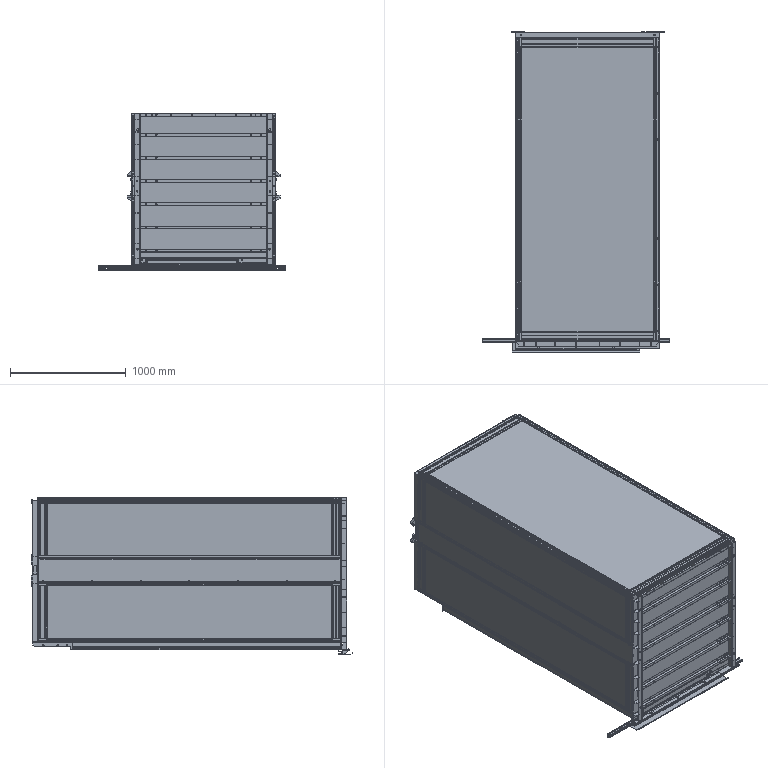Part | 170 solids | 7270 faces | volume 150842549 mm3 | plane 4451 | cylinder 2735 | cone 72 | spline 12 | commonest cylinder face diameters 0.6 x312 0.4 x308 11 x211 10 x208 13 x204 9 x182